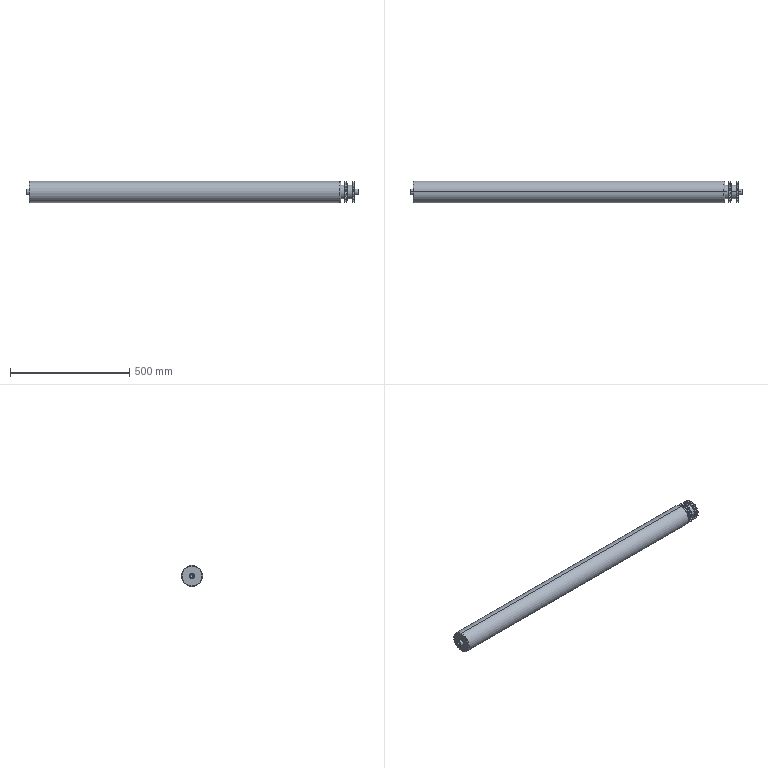Part | SolidWorks | features MoveFace 11, ICE 8, HoleWzd 3, BaseBody 1, Chamfer 1 | 1 solid | 228 faces | box 1393 x 89 x 89 mm | volume 8327886 mm3 | cylinder 148 | torus 68 | plane 8 | cone 4 | commonest cylinder face diameters 41.452 x62 10.262 x42 86.038 x30 14 x4 25 x4 58 x4